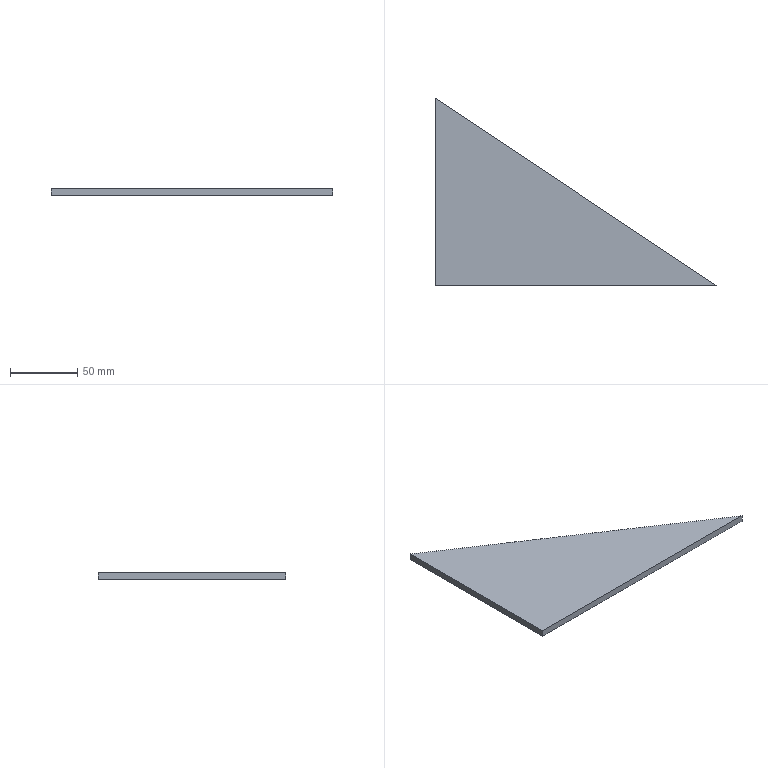Part | SolidWorks | features FlatPattern 1, SMBaseFlange 1, SheetMetal 1 | 1 solid | 5 faces | box 210 x 140 x 5 mm | volume 73500 mm3 | plane 5
STEP:
#1=CARTESIAN_POINT('',(210.,0.,0.));
#2=VERTEX_POINT('',#1);
#3=CARTESIAN_POINT('',(0.,140.,0.));
#4=VERTEX_POINT('',#3);
#5=CARTESIAN_POINT('',(210.,0.,0.));
#6=DIRECTION('',(-0.8321,0.5547,0.));
#7=VECTOR('',#6,1000.);
#8=LINE('',#5,#7);
#9=EDGE_CURVE('',#2,#4,#8,.T.);
#10=ORIENTED_EDGE('',*,*,#9,.F.);
#11=CARTESIAN_POINT('',(210.,0.,-5.));
#12=VERTEX_POINT('',#11);
#13=CARTESIAN_POINT('',(210.,0.,-5.));
#14=DIRECTION('',(0.,0.,1.));
#15=VECTOR('',#14,1000.);
#16=LINE('',#13,#15);
#17=EDGE_CURVE('',#12,#2,#16,.T.);
#18=ORIENTED_EDGE('',*,*,#17,.F.);
#19=CARTESIAN_POINT('',(0.,140.,-5.));
#20=VERTEX_POINT('',#19);
#21=CARTESIAN_POINT('',(210.,0.,-5.));
#22=DIRECTION('',(-0.8321,0.5547,0.));
#23=VECTOR('',#22,1000.);
#24=LINE('',#21,#23);
#25=EDGE_CURVE('',#12,#20,#24,.T.);
#26=ORIENTED_EDGE('',*,*,#25,.T.);
#27=CARTESIAN_POINT('',(0.,140.,-5.));
#28=DIRECTION('',(0.,0.,1.));
#29=VECTOR('',#28,1000.);
#30=LINE('',#27,#29);
#31=EDGE_CURVE('',#20,#4,#30,.T.);
#32=ORIENTED_EDGE('',*,*,#31,.T.);
#33=EDGE_LOOP('',(#10,#18,#26,#32));
#34=FACE_OUTER_BOUND('',#33,.T.);
#35=CARTESIAN_POINT('',(210.,0.,-5.));
#36=DIRECTION('',(0.5547,0.8321,0.));
#37=DIRECTION('',(-0.8321,0.5547,0.));
#38=AXIS2_PLACEMENT_3D('',#35,#36,#37);
#39=PLANE('',#38);
#40=ADVANCED_FACE('',(#34),#39,.T.);
#41=CARTESIAN_POINT('',(0.,0.,0.));
#42=VERTEX_POINT('',#41);
#43=CARTESIAN_POINT('',(0.,0.,0.));
#44=DIRECTION('',(1.,0.,0.));
#45=VECTOR('',#44,1000.);
#46=LINE('',#43,#45);
#47=EDGE_CURVE('',#42,#2,#46,.T.);
#48=ORIENTED_EDGE('',*,*,#47,.F.);
#49=CARTESIAN_POINT('',(0.,0.,-5.));
#50=VERTEX_POINT('',#49);
#51=CARTESIAN_POINT('',(0.,0.,-5.));
#52=DIRECTION('',(0.,0.,1.));
#53=VECTOR('',#52,1000.);
#54=LINE('',#51,#53);
#55=EDGE_CURVE('',#50,#42,#54,.T.);
#56=ORIENTED_EDGE('',*,*,#55,.F.);
#57=CARTESIAN_POINT('',(0.,0.,-5.));
#58=DIRECTION('',(1.,0.,0.));
#59=VECTOR('',#58,1000.);
#60=LINE('',#57,#59);
#61=EDGE_CURVE('',#50,#12,#60,.T.);
#62=ORIENTED_EDGE('',*,*,#61,.T.);
#63=ORIENTED_EDGE('',*,*,#17,.T.);
#64=EDGE_LOOP('',(#48,#56,#62,#63));
#65=FACE_OUTER_BOUND('',#64,.T.);
#66=CARTESIAN_POINT('',(0.,0.,-5.));
#67=DIRECTION('',(0.,-1.,0.));
#68=DIRECTION('',(0.,0.,-1.));
#69=AXIS2_PLACEMENT_3D('',#66,#67,#68);
#70=PLANE('',#69);
#71=ADVANCED_FACE('',(#65),#70,.T.);
#72=CARTESIAN_POINT('',(0.,140.,0.));
#73=DIRECTION('',(0.,-1.,0.));
#74=VECTOR('',#73,1000.);
#75=LINE('',#72,#74);
#76=EDGE_CURVE('',#4,#42,#75,.T.);
#77=ORIENTED_EDGE('',*,*,#76,.F.);
#78=ORIENTED_EDGE('',*,*,#31,.F.);
#79=CARTESIAN_POINT('',(0.,140.,-5.));
#80=DIRECTION('',(0.,-1.,0.));
#81=VECTOR('',#80,1000.);
#82=LINE('',#79,#81);
#83=EDGE_CURVE('',#20,#50,#82,.T.);
#84=ORIENTED_EDGE('',*,*,#83,.T.);
#85=ORIENTED_EDGE('',*,*,#55,.T.);
#86=EDGE_LOOP('',(#77,#78,#84,#85));
#87=FACE_OUTER_BOUND('',#86,.T.);
#88=CARTESIAN_POINT('',(0.,140.,-5.));
#89=DIRECTION('',(-1.,0.,0.));
#90=DIRECTION('',(0.,-1.,0.));
#91=AXIS2_PLACEMENT_3D('',#88,#89,#90);
#92=PLANE('',#91);
#93=ADVANCED_FACE('',(#87),#92,.T.);
#94=ORIENTED_EDGE('',*,*,#25,.F.);
#95=ORIENTED_EDGE('',*,*,#61,.F.);
#96=ORIENTED_EDGE('',*,*,#83,.F.);
#97=EDGE_LOOP('',(#94,#95,#96));
#98=FACE_OUTER_BOUND('',#97,.T.);
#99=CARTESIAN_POINT('',(0.,0.,-5.));
#100=DIRECTION('',(0.,0.,1.));
#101=DIRECTION('',(1.,0.,0.));
#102=AXIS2_PLACEMENT_3D('',#99,#100,#101);
#103=PLANE('',#102);
#104=ADVANCED_FACE('',(#98),#103,.F.);
#105=ORIENTED_EDGE('',*,*,#9,.T.);
#106=ORIENTED_EDGE('',*,*,#76,.T.);
#107=ORIENTED_EDGE('',*,*,#47,.T.);
#108=EDGE_LOOP('',(#105,#106,#107));
#109=FACE_OUTER_BOUND('',#108,.T.);
#110=CARTESIAN_POINT('',(0.,0.,0.));
#111=DIRECTION('',(0.,0.,1.));
#112=DIRECTION('',(1.,0.,0.));
#113=AXIS2_PLACEMENT_3D('',#110,#111,#112);
#114=PLANE('',#113);
#115=ADVANCED_FACE('',(#109),#114,.T.);
#116=CLOSED_SHELL('',(#40,#71,#93,#104,#115));
#117=MANIFOLD_SOLID_BREP('',#116);
#118=CARTESIAN_POINT('',(0.,0.,0.));
#119=DIRECTION('',(0.,0.,1.));
#120=DIRECTION('',(1.,0.,0.));
#121=AXIS2_PLACEMENT_3D('',#118,#119,#120);
#122=(LENGTH_UNIT()NAMED_UNIT(*)SI_UNIT(.MILLI.,.METRE.));
#123=UNCERTAINTY_MEASURE_WITH_UNIT(LENGTH_MEASURE(0.00001),#122,'','');
#124=(NAMED_UNIT(*)PLANE_ANGLE_UNIT()SI_UNIT($,.RADIAN.));
#125=(NAMED_UNIT(*)SI_UNIT($,.STERADIAN.)SOLID_ANGLE_UNIT());
#126=(GEOMETRIC_REPRESENTATION_CONTEXT(3)GLOBAL_UNCERTAINTY_ASSIGNED_CONTEXT((#123))GLOBAL_UNIT_ASSIGNED_CONTEXT((#122,#124,#125))REPRESENTATION_CONTEXT('',''));
#127=ADVANCED_BREP_SHAPE_REPRESENTATION('',(#117,#121),#126);